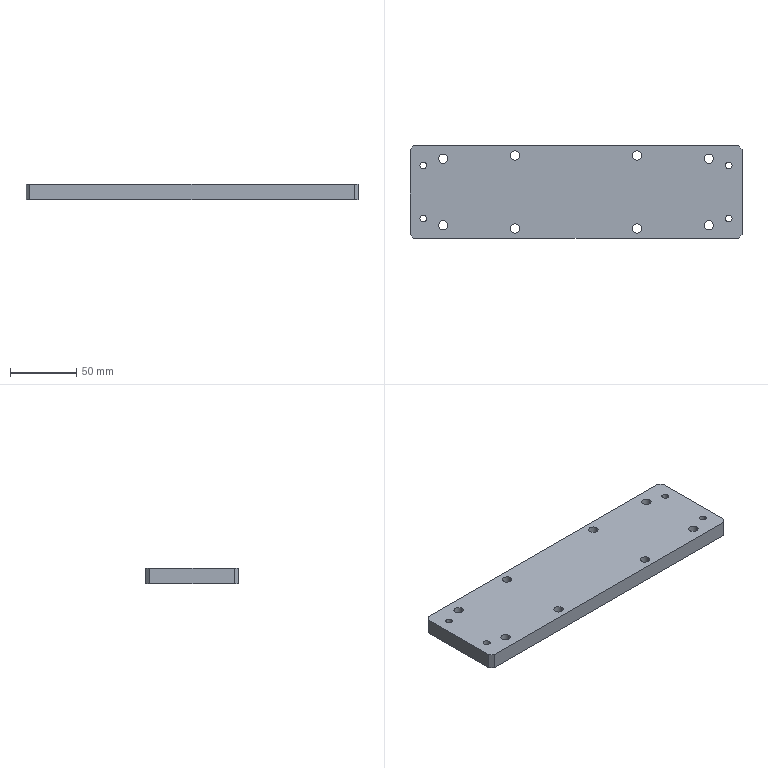Part | SolidWorks | features HoleWzd 3, Chamfer 1, Extrusion 1 | 1 solid | 34 faces | box 250 x 70 x 12 mm | volume 205147 mm3 | cylinder 24 | plane 10 | commonest cylinder face diameters 7 x16 5 x8
STEP:
#1=CARTESIAN_POINT('',(-42.5,27.5,12.));
#2=VERTEX_POINT('',#1);
#3=CARTESIAN_POINT('',(-49.5,27.5,12.));
#4=VERTEX_POINT('',#3);
#5=CARTESIAN_POINT('',(-46.,27.5,12.));
#6=DIRECTION('',(0.,0.,-1.));
#7=DIRECTION('',(-1.,0.,0.));
#8=AXIS2_PLACEMENT_3D('',#5,#6,#7);
#9=CIRCLE('',#8,3.5);
#10=EDGE_CURVE('',#2,#4,#9,.T.);
#11=ORIENTED_EDGE('',*,*,#10,.F.);
#12=CARTESIAN_POINT('',(-42.5,27.5,0.));
#13=VERTEX_POINT('',#12);
#14=CARTESIAN_POINT('',(-42.5,27.5,0.));
#15=DIRECTION('',(0.,0.,-1.));
#16=VECTOR('',#15,1000.);
#17=LINE('',#14,#16);
#18=EDGE_CURVE('',#2,#13,#17,.T.);
#19=ORIENTED_EDGE('',*,*,#18,.T.);
#20=CARTESIAN_POINT('',(-49.5,27.5,0.));
#21=VERTEX_POINT('',#20);
#22=CARTESIAN_POINT('',(-46.,27.5,0.));
#23=DIRECTION('',(0.,0.,-1.));
#24=DIRECTION('',(-1.,0.,0.));
#25=AXIS2_PLACEMENT_3D('',#22,#23,#24);
#26=CIRCLE('',#25,3.5);
#27=EDGE_CURVE('',#13,#21,#26,.T.);
#28=ORIENTED_EDGE('',*,*,#27,.T.);
#29=CARTESIAN_POINT('',(-49.5,27.5,0.));
#30=DIRECTION('',(0.,0.,-1.));
#31=VECTOR('',#30,1000.);
#32=LINE('',#29,#31);
#33=EDGE_CURVE('',#4,#21,#32,.T.);
#34=ORIENTED_EDGE('',*,*,#33,.F.);
#35=EDGE_LOOP('',(#11,#19,#28,#34));
#36=FACE_OUTER_BOUND('',#35,.T.);
#37=CARTESIAN_POINT('',(-46.,27.5,0.));
#38=DIRECTION('',(0.,0.,-1.));
#39=DIRECTION('',(-1.,0.,0.));
#40=AXIS2_PLACEMENT_3D('',#37,#38,#39);
#41=CYLINDRICAL_SURFACE('',#40,3.5);
#42=ADVANCED_FACE('',(#36),#41,.F.);
#43=CARTESIAN_POINT('',(-42.5,-27.5,12.));
#44=VERTEX_POINT('',#43);
#45=CARTESIAN_POINT('',(-49.5,-27.5,12.));
#46=VERTEX_POINT('',#45);
#47=CARTESIAN_POINT('',(-46.,-27.5,12.));
#48=DIRECTION('',(0.,0.,-1.));
#49=DIRECTION('',(-1.,0.,0.));
#50=AXIS2_PLACEMENT_3D('',#47,#48,#49);
#51=CIRCLE('',#50,3.5);
#52=EDGE_CURVE('',#44,#46,#51,.T.);
#53=ORIENTED_EDGE('',*,*,#52,.F.);
#54=CARTESIAN_POINT('',(-42.5,-27.5,0.));
#55=VERTEX_POINT('',#54);
#56=CARTESIAN_POINT('',(-42.5,-27.5,0.));
#57=DIRECTION('',(0.,0.,-1.));
#58=VECTOR('',#57,1000.);
#59=LINE('',#56,#58);
#60=EDGE_CURVE('',#44,#55,#59,.T.);
#61=ORIENTED_EDGE('',*,*,#60,.T.);
#62=CARTESIAN_POINT('',(-49.5,-27.5,0.));
#63=VERTEX_POINT('',#62);
#64=CARTESIAN_POINT('',(-46.,-27.5,0.));
#65=DIRECTION('',(0.,0.,-1.));
#66=DIRECTION('',(-1.,0.,0.));
#67=AXIS2_PLACEMENT_3D('',#64,#65,#66);
#68=CIRCLE('',#67,3.5);
#69=EDGE_CURVE('',#55,#63,#68,.T.);
#70=ORIENTED_EDGE('',*,*,#69,.T.);
#71=CARTESIAN_POINT('',(-49.5,-27.5,0.));
#72=DIRECTION('',(0.,0.,-1.));
#73=VECTOR('',#72,1000.);
#74=LINE('',#71,#73);
#75=EDGE_CURVE('',#46,#63,#74,.T.);
#76=ORIENTED_EDGE('',*,*,#75,.F.);
#77=EDGE_LOOP('',(#53,#61,#70,#76));
#78=FACE_OUTER_BOUND('',#77,.T.);
#79=CARTESIAN_POINT('',(-46.,-27.5,0.));
#80=DIRECTION('',(0.,0.,-1.));
#81=DIRECTION('',(-1.,0.,0.));
#82=AXIS2_PLACEMENT_3D('',#79,#80,#81);
#83=CYLINDRICAL_SURFACE('',#82,3.5);
#84=ADVANCED_FACE('',(#78),#83,.F.);
#85=CARTESIAN_POINT('',(49.5,27.5,12.));
#86=VERTEX_POINT('',#85);
#87=CARTESIAN_POINT('',(42.5,27.5,12.));
#88=VERTEX_POINT('',#87);
#89=CARTESIAN_POINT('',(46.,27.5,12.));
#90=DIRECTION('',(0.,0.,-1.));
#91=DIRECTION('',(-1.,0.,0.));
#92=AXIS2_PLACEMENT_3D('',#89,#90,#91);
#93=CIRCLE('',#92,3.5);
#94=EDGE_CURVE('',#86,#88,#93,.T.);
#95=ORIENTED_EDGE('',*,*,#94,.F.);
#96=CARTESIAN_POINT('',(49.5,27.5,0.));
#97=VERTEX_POINT('',#96);
#98=CARTESIAN_POINT('',(49.5,27.5,0.));
#99=DIRECTION('',(0.,0.,-1.));
#100=VECTOR('',#99,1000.);
#101=LINE('',#98,#100);
#102=EDGE_CURVE('',#86,#97,#101,.T.);
#103=ORIENTED_EDGE('',*,*,#102,.T.);
#104=CARTESIAN_POINT('',(42.5,27.5,0.));
#105=VERTEX_POINT('',#104);
#106=CARTESIAN_POINT('',(46.,27.5,0.));
#107=DIRECTION('',(0.,0.,-1.));
#108=DIRECTION('',(-1.,0.,0.));
#109=AXIS2_PLACEMENT_3D('',#106,#107,#108);
#110=CIRCLE('',#109,3.5);
#111=EDGE_CURVE('',#97,#105,#110,.T.);
#112=ORIENTED_EDGE('',*,*,#111,.T.);
#113=CARTESIAN_POINT('',(42.5,27.5,0.));
#114=DIRECTION('',(0.,0.,-1.));
#115=VECTOR('',#114,1000.);
#116=LINE('',#113,#115);
#117=EDGE_CURVE('',#88,#105,#116,.T.);
#118=ORIENTED_EDGE('',*,*,#117,.F.);
#119=EDGE_LOOP('',(#95,#103,#112,#118));
#120=FACE_OUTER_BOUND('',#119,.T.);
#121=CARTESIAN_POINT('',(46.,27.5,0.));
#122=DIRECTION('',(0.,0.,-1.));
#123=DIRECTION('',(-1.,0.,0.));
#124=AXIS2_PLACEMENT_3D('',#121,#122,#123);
#125=CYLINDRICAL_SURFACE('',#124,3.5);
#126=ADVANCED_FACE('',(#120),#125,.F.);
#127=CARTESIAN_POINT('',(49.5,-27.5,12.));
#128=VERTEX_POINT('',#127);
#129=CARTESIAN_POINT('',(42.5,-27.5,12.));
#130=VERTEX_POINT('',#129);
#131=CARTESIAN_POINT('',(46.,-27.5,12.));
#132=DIRECTION('',(0.,0.,-1.));
#133=DIRECTION('',(-1.,0.,0.));
#134=AXIS2_PLACEMENT_3D('',#131,#132,#133);
#135=CIRCLE('',#134,3.5);
#136=EDGE_CURVE('',#128,#130,#135,.T.);
#137=ORIENTED_EDGE('',*,*,#136,.F.);
#138=CARTESIAN_POINT('',(49.5,-27.5,0.));
#139=VERTEX_POINT('',#138);
#140=CARTESIAN_POINT('',(49.5,-27.5,0.));
#141=DIRECTION('',(0.,0.,-1.));
#142=VECTOR('',#141,1000.);
#143=LINE('',#140,#142);
#144=EDGE_CURVE('',#128,#139,#143,.T.);
#145=ORIENTED_EDGE('',*,*,#144,.T.);
#146=CARTESIAN_POINT('',(42.5,-27.5,0.));
#147=VERTEX_POINT('',#146);
#148=CARTESIAN_POINT('',(46.,-27.5,0.));
#149=DIRECTION('',(0.,0.,-1.));
#150=DIRECTION('',(-1.,0.,0.));
#151=AXIS2_PLACEMENT_3D('',#148,#149,#150);
#152=CIRCLE('',#151,3.5);
#153=EDGE_CURVE('',#139,#147,#152,.T.);
#154=ORIENTED_EDGE('',*,*,#153,.T.);
#155=CARTESIAN_POINT('',(42.5,-27.5,0.));
#156=DIRECTION('',(0.,0.,-1.));
#157=VECTOR('',#156,1000.);
#158=LINE('',#155,#157);
#159=EDGE_CURVE('',#130,#147,#158,.T.);
#160=ORIENTED_EDGE('',*,*,#159,.F.);
#161=EDGE_LOOP('',(#137,#145,#154,#160));
#162=FACE_OUTER_BOUND('',#161,.T.);
#163=CARTESIAN_POINT('',(46.,-27.5,0.));
#164=DIRECTION('',(0.,0.,-1.));
#165=DIRECTION('',(-1.,0.,0.));
#166=AXIS2_PLACEMENT_3D('',#163,#164,#165);
#167=CYLINDRICAL_SURFACE('',#166,3.5);
#168=ADVANCED_FACE('',(#162),#167,.F.);
#169=CARTESIAN_POINT('',(-112.5,-20.,12.));
#170=VERTEX_POINT('',#169);
#171=CARTESIAN_POINT('',(-117.5,-20.,12.));
#172=VERTEX_POINT('',#171);
#173=CARTESIAN_POINT('',(-115.,-20.,12.));
#174=DIRECTION('',(0.,0.,-1.));
#175=DIRECTION('',(-1.,0.,0.));
#176=AXIS2_PLACEMENT_3D('',#173,#174,#175);
#177=CIRCLE('',#176,2.5);
#178=EDGE_CURVE('',#170,#172,#177,.T.);
#179=ORIENTED_EDGE('',*,*,#178,.F.);
#180=CARTESIAN_POINT('',(-112.5,-20.,0.));
#181=VERTEX_POINT('',#180);
#182=CARTESIAN_POINT('',(-112.5,-20.,0.));
#183=DIRECTION('',(0.,0.,-1.));
#184=VECTOR('',#183,1000.);
#185=LINE('',#182,#184);
#186=EDGE_CURVE('',#170,#181,#185,.T.);
#187=ORIENTED_EDGE('',*,*,#186,.T.);
#188=CARTESIAN_POINT('',(-117.5,-20.,0.));
#189=VERTEX_POINT('',#188);
#190=CARTESIAN_POINT('',(-115.,-20.,0.));
#191=DIRECTION('',(0.,0.,-1.));
#192=DIRECTION('',(-1.,0.,0.));
#193=AXIS2_PLACEMENT_3D('',#190,#191,#192);
#194=CIRCLE('',#193,2.5);
#195=EDGE_CURVE('',#181,#189,#194,.T.);
#196=ORIENTED_EDGE('',*,*,#195,.T.);
#197=CARTESIAN_POINT('',(-117.5,-20.,0.));
#198=DIRECTION('',(0.,0.,-1.));
#199=VECTOR('',#198,1000.);
#200=LINE('',#197,#199);
#201=EDGE_CURVE('',#172,#189,#200,.T.);
#202=ORIENTED_EDGE('',*,*,#201,.F.);
#203=EDGE_LOOP('',(#179,#187,#196,#202));
#204=FACE_OUTER_BOUND('',#203,.T.);
#205=CARTESIAN_POINT('',(-115.,-20.,0.));
#206=DIRECTION('',(0.,0.,-1.));
#207=DIRECTION('',(-1.,0.,0.));
#208=AXIS2_PLACEMENT_3D('',#205,#206,#207);
#209=CYLINDRICAL_SURFACE('',#208,2.5);
#210=ADVANCED_FACE('',(#204),#209,.F.);
#211=CARTESIAN_POINT('',(-112.5,20.,12.));
#212=VERTEX_POINT('',#211);
#213=CARTESIAN_POINT('',(-117.5,20.,12.));
#214=VERTEX_POINT('',#213);
#215=CARTESIAN_POINT('',(-115.,20.,12.));
#216=DIRECTION('',(0.,0.,-1.));
#217=DIRECTION('',(-1.,0.,0.));
#218=AXIS2_PLACEMENT_3D('',#215,#216,#217);
#219=CIRCLE('',#218,2.5);
#220=EDGE_CURVE('',#212,#214,#219,.T.);
#221=ORIENTED_EDGE('',*,*,#220,.F.);
#222=CARTESIAN_POINT('',(-112.5,20.,0.));
#223=VERTEX_POINT('',#222);
#224=CARTESIAN_POINT('',(-112.5,20.,0.));
#225=DIRECTION('',(0.,0.,-1.));
#226=VECTOR('',#225,1000.);
#227=LINE('',#224,#226);
#228=EDGE_CURVE('',#212,#223,#227,.T.);
#229=ORIENTED_EDGE('',*,*,#228,.T.);
#230=CARTESIAN_POINT('',(-117.5,20.,0.));
#231=VERTEX_POINT('',#230);
#232=CARTESIAN_POINT('',(-115.,20.,0.));
#233=DIRECTION('',(0.,0.,-1.));
#234=DIRECTION('',(-1.,0.,0.));
#235=AXIS2_PLACEMENT_3D('',#232,#233,#234);
#236=CIRCLE('',#235,2.5);
#237=EDGE_CURVE('',#223,#231,#236,.T.);
#238=ORIENTED_EDGE('',*,*,#237,.T.);
#239=CARTESIAN_POINT('',(-117.5,20.,0.));
#240=DIRECTION('',(0.,0.,-1.));
#241=VECTOR('',#240,1000.);
#242=LINE('',#239,#241);
#243=EDGE_CURVE('',#214,#231,#242,.T.);
#244=ORIENTED_EDGE('',*,*,#243,.F.);
#245=EDGE_LOOP('',(#221,#229,#238,#244));
#246=FACE_OUTER_BOUND('',#245,.T.);
#247=CARTESIAN_POINT('',(-115.,20.,0.));
#248=DIRECTION('',(0.,0.,-1.));
#249=DIRECTION('',(-1.,0.,0.));
#250=AXIS2_PLACEMENT_3D('',#247,#248,#249);
#251=CYLINDRICAL_SURFACE('',#250,2.5);
#252=ADVANCED_FACE('',(#246),#251,.F.);
#253=CARTESIAN_POINT('',(117.5,20.,12.));
#254=VERTEX_POINT('',#253);
#255=CARTESIAN_POINT('',(112.5,20.,12.));
#256=VERTEX_POINT('',#255);
#257=CARTESIAN_POINT('',(115.,20.,12.));
#258=DIRECTION('',(0.,0.,-1.));
#259=DIRECTION('',(-1.,0.,0.));
#260=AXIS2_PLACEMENT_3D('',#257,#258,#259);
#261=CIRCLE('',#260,2.5);
#262=EDGE_CURVE('',#254,#256,#261,.T.);
#263=ORIENTED_EDGE('',*,*,#262,.F.);
#264=CARTESIAN_POINT('',(117.5,20.,0.));
#265=VERTEX_POINT('',#264);
#266=CARTESIAN_POINT('',(117.5,20.,0.));
#267=DIRECTION('',(0.,0.,-1.));
#268=VECTOR('',#267,1000.);
#269=LINE('',#266,#268);
#270=EDGE_CURVE('',#254,#265,#269,.T.);
#271=ORIENTED_EDGE('',*,*,#270,.T.);
#272=CARTESIAN_POINT('',(112.5,20.,0.));
#273=VERTEX_POINT('',#272);
#274=CARTESIAN_POINT('',(115.,20.,0.));
#275=DIRECTION('',(0.,0.,-1.));
#276=DIRECTION('',(-1.,0.,0.));
#277=AXIS2_PLACEMENT_3D('',#274,#275,#276);
#278=CIRCLE('',#277,2.5);
#279=EDGE_CURVE('',#265,#273,#278,.T.);
#280=ORIENTED_EDGE('',*,*,#279,.T.);
#281=CARTESIAN_POINT('',(112.5,20.,0.));
#282=DIRECTION('',(0.,0.,-1.));
#283=VECTOR('',#282,1000.);
#284=LINE('',#281,#283);
#285=EDGE_CURVE('',#256,#273,#284,.T.);
#286=ORIENTED_EDGE('',*,*,#285,.F.);
#287=EDGE_LOOP('',(#263,#271,#280,#286));
#288=FACE_OUTER_BOUND('',#287,.T.);
#289=CARTESIAN_POINT('',(115.,20.,0.));
#290=DIRECTION('',(0.,0.,-1.));
#291=DIRECTION('',(-1.,0.,0.));
#292=AXIS2_PLACEMENT_3D('',#289,#290,#291);
#293=CYLINDRICAL_SURFACE('',#292,2.5);
#294=ADVANCED_FACE('',(#288),#293,.F.);
#295=CARTESIAN_POINT('',(117.5,-20.,12.));
#296=VERTEX_POINT('',#295);
#297=CARTESIAN_POINT('',(112.5,-20.,12.));
#298=VERTEX_POINT('',#297);
#299=CARTESIAN_POINT('',(115.,-20.,12.));
#300=DIRECTION('',(0.,0.,-1.));
#301=DIRECTION('',(-1.,0.,0.));
#302=AXIS2_PLACEMENT_3D('',#299,#300,#301);
#303=CIRCLE('',#302,2.5);
#304=EDGE_CURVE('',#296,#298,#303,.T.);
#305=ORIENTED_EDGE('',*,*,#304,.F.);
#306=CARTESIAN_POINT('',(117.5,-20.,0.));
#307=VERTEX_POINT('',#306);
#308=CARTESIAN_POINT('',(117.5,-20.,0.));
#309=DIRECTION('',(0.,0.,-1.));
#310=VECTOR('',#309,1000.);
#311=LINE('',#308,#310);
#312=EDGE_CURVE('',#296,#307,#311,.T.);
#313=ORIENTED_EDGE('',*,*,#312,.T.);
#314=CARTESIAN_POINT('',(112.5,-20.,0.));
#315=VERTEX_POINT('',#314);
#316=CARTESIAN_POINT('',(115.,-20.,0.));
#317=DIRECTION('',(0.,0.,-1.));
#318=DIRECTION('',(-1.,0.,0.));
#319=AXIS2_PLACEMENT_3D('',#316,#317,#318);
#320=CIRCLE('',#319,2.5);
#321=EDGE_CURVE('',#307,#315,#320,.T.);
#322=ORIENTED_EDGE('',*,*,#321,.T.);
#323=CARTESIAN_POINT('',(112.5,-20.,0.));
#324=DIRECTION('',(0.,0.,-1.));
#325=VECTOR('',#324,1000.);
#326=LINE('',#323,#325);
#327=EDGE_CURVE('',#298,#315,#326,.T.);
#328=ORIENTED_EDGE('',*,*,#327,.F.);
#329=EDGE_LOOP('',(#305,#313,#322,#328));
#330=FACE_OUTER_BOUND('',#329,.T.);
#331=CARTESIAN_POINT('',(115.,-20.,0.));
#332=DIRECTION('',(0.,0.,-1.));
#333=DIRECTION('',(-1.,0.,0.));
#334=AXIS2_PLACEMENT_3D('',#331,#332,#333);
#335=CYLINDRICAL_SURFACE('',#334,2.5);
#336=ADVANCED_FACE('',(#330),#335,.F.);
#337=CARTESIAN_POINT('',(-96.5,-25.,12.));
#338=VERTEX_POINT('',#337);
#339=CARTESIAN_POINT('',(-103.5,-25.,12.));
#340=VERTEX_POINT('',#339);
#341=CARTESIAN_POINT('',(-100.,-25.,12.));
#342=DIRECTION('',(0.,0.,-1.));
#343=DIRECTION('',(-1.,0.,0.));
#344=AXIS2_PLACEMENT_3D('',#341,#342,#343);
#345=CIRCLE('',#344,3.5);
#346=EDGE_CURVE('',#338,#340,#345,.T.);
#347=ORIENTED_EDGE('',*,*,#346,.F.);
#348=CARTESIAN_POINT('',(-96.5,-25.,0.));
#349=VERTEX_POINT('',#348);
#350=CARTESIAN_POINT('',(-96.5,-25.,0.));
#351=DIRECTION('',(0.,0.,-1.));
#352=VECTOR('',#351,1000.);
#353=LINE('',#350,#352);
#354=EDGE_CURVE('',#338,#349,#353,.T.);
#355=ORIENTED_EDGE('',*,*,#354,.T.);
#356=CARTESIAN_POINT('',(-103.5,-25.,0.));
#357=VERTEX_POINT('',#356);
#358=CARTESIAN_POINT('',(-100.,-25.,0.));
#359=DIRECTION('',(0.,0.,-1.));
#360=DIRECTION('',(-1.,0.,0.));
#361=AXIS2_PLACEMENT_3D('',#358,#359,#360);
#362=CIRCLE('',#361,3.5);
#363=EDGE_CURVE('',#349,#357,#362,.T.);
#364=ORIENTED_EDGE('',*,*,#363,.T.);
#365=CARTESIAN_POINT('',(-103.5,-25.,0.));
#366=DIRECTION('',(0.,0.,-1.));
#367=VECTOR('',#366,1000.);
#368=LINE('',#365,#367);
#369=EDGE_CURVE('',#340,#357,#368,.T.);
#370=ORIENTED_EDGE('',*,*,#369,.F.);
#371=EDGE_LOOP('',(#347,#355,#364,#370));
#372=FACE_OUTER_BOUND('',#371,.T.);
#373=CARTESIAN_POINT('',(-100.,-25.,0.));
#374=DIRECTION('',(0.,0.,-1.));
#375=DIRECTION('',(-1.,0.,0.));
#376=AXIS2_PLACEMENT_3D('',#373,#374,#375);
#377=CYLINDRICAL_SURFACE('',#376,3.5);
#378=ADVANCED_FACE('',(#372),#377,.F.);
#379=CARTESIAN_POINT('',(-96.5,25.,12.));
#380=VERTEX_POINT('',#379);
#381=CARTESIAN_POINT('',(-103.5,25.,12.));
#382=VERTEX_POINT('',#381);
#383=CARTESIAN_POINT('',(-100.,25.,12.));
#384=DIRECTION('',(0.,0.,-1.));
#385=DIRECTION('',(-1.,0.,0.));
#386=AXIS2_PLACEMENT_3D('',#383,#384,#385);
#387=CIRCLE('',#386,3.5);
#388=EDGE_CURVE('',#380,#382,#387,.T.);
#389=ORIENTED_EDGE('',*,*,#388,.F.);
#390=CARTESIAN_POINT('',(-96.5,25.,0.));
#391=VERTEX_POINT('',#390);
#392=CARTESIAN_POINT('',(-96.5,25.,0.));
#393=DIRECTION('',(0.,0.,-1.));
#394=VECTOR('',#393,1000.);
#395=LINE('',#392,#394);
#396=EDGE_CURVE('',#380,#391,#395,.T.);
#397=ORIENTED_EDGE('',*,*,#396,.T.);
#398=CARTESIAN_POINT('',(-103.5,25.,0.));
#399=VERTEX_POINT('',#398);
#400=CARTESIAN_POINT('',(-100.,25.,0.));
#401=DIRECTION('',(0.,0.,-1.));
#402=DIRECTION('',(-1.,0.,0.));
#403=AXIS2_PLACEMENT_3D('',#400,#401,#402);
#404=CIRCLE('',#403,3.5);
#405=EDGE_CURVE('',#391,#399,#404,.T.);
#406=ORIENTED_EDGE('',*,*,#405,.T.);
#407=CARTESIAN_POINT('',(-103.5,25.,0.));
#408=DIRECTION('',(0.,0.,-1.));
#409=VECTOR('',#408,1000.);
#410=LINE('',#407,#409);
#411=EDGE_CURVE('',#382,#399,#410,.T.);
#412=ORIENTED_EDGE('',*,*,#411,.F.);
#413=EDGE_LOOP('',(#389,#397,#406,#412));
#414=FACE_OUTER_BOUND('',#413,.T.);
#415=CARTESIAN_POINT('',(-100.,25.,0.));
#416=DIRECTION('',(0.,0.,-1.));
#417=DIRECTION('',(-1.,0.,0.));
#418=AXIS2_PLACEMENT_3D('',#415,#416,#417);
#419=CYLINDRICAL_SURFACE('',#418,3.5);
#420=ADVANCED_FACE('',(#414),#419,.F.);
#421=CARTESIAN_POINT('',(103.5,25.,12.));
#422=VERTEX_POINT('',#421);
#423=CARTESIAN_POINT('',(96.5,25.,12.));
#424=VERTEX_POINT('',#423);
#425=CARTESIAN_POINT('',(100.,25.,12.));
#426=DIRECTION('',(0.,0.,-1.));
#427=DIRECTION('',(-1.,0.,0.));
#428=AXIS2_PLACEMENT_3D('',#425,#426,#427);
#429=CIRCLE('',#428,3.5);
#430=EDGE_CURVE('',#422,#424,#429,.T.);
#431=ORIENTED_EDGE('',*,*,#430,.F.);
#432=CARTESIAN_POINT('',(103.5,25.,0.));
#433=VERTEX_POINT('',#432);
#434=CARTESIAN_POINT('',(103.5,25.,0.));
#435=DIRECTION('',(0.,0.,-1.));
#436=VECTOR('',#435,1000.);
#437=LINE('',#434,#436);
#438=EDGE_CURVE('',#422,#433,#437,.T.);
#439=ORIENTED_EDGE('',*,*,#438,.T.);
#440=CARTESIAN_POINT('',(96.5,25.,0.));
#441=VERTEX_POINT('',#440);
#442=CARTESIAN_POINT('',(100.,25.,0.));
#443=DIRECTION('',(0.,0.,-1.));
#444=DIRECTION('',(-1.,0.,0.));
#445=AXIS2_PLACEMENT_3D('',#442,#443,#444);
#446=CIRCLE('',#445,3.5);
#447=EDGE_CURVE('',#433,#441,#446,.T.);
#448=ORIENTED_EDGE('',*,*,#447,.T.);
#449=CARTESIAN_POINT('',(96.5,25.,0.));
#450=DIRECTION('',(0.,0.,-1.));
#451=VECTOR('',#450,1000.);
#452=LINE('',#449,#451);
#453=EDGE_CURVE('',#424,#441,#452,.T.);
#454=ORIENTED_EDGE('',*,*,#453,.F.);
#455=EDGE_LOOP('',(#431,#439,#448,#454));
#456=FACE_OUTER_BOUND('',#455,.T.);
#457=CARTESIAN_POINT('',(100.,25.,0.));
#458=DIRECTION('',(0.,0.,-1.));
#459=DIRECTION('',(-1.,0.,0.));
#460=AXIS2_PLACEMENT_3D('',#457,#458,#459);
#461=CYLINDRICAL_SURFACE('',#460,3.5);
#462=ADVANCED_FACE('',(#456),#461,.F.);
#463=CARTESIAN_POINT('',(103.5,-25.,12.));
#464=VERTEX_POINT('',#463);
#465=CARTESIAN_POINT('',(96.5,-25.,12.));
#466=VERTEX_POINT('',#465);
#467=CARTESIAN_POINT('',(100.,-25.,12.));
#468=DIRECTION('',(0.,0.,-1.));
#469=DIRECTION('',(-1.,0.,0.));
#470=AXIS2_PLACEMENT_3D('',#467,#468,#469);
#471=CIRCLE('',#470,3.5);
#472=EDGE_CURVE('',#464,#466,#471,.T.);
#473=ORIENTED_EDGE('',*,*,#472,.F.);
#474=CARTESIAN_POINT('',(103.5,-25.,0.));
#475=VERTEX_POINT('',#474);
#476=CARTESIAN_POINT('',(103.5,-25.,0.));
#477=DIRECTION('',(0.,0.,-1.));
#478=VECTOR('',#477,1000.);
#479=LINE('',#476,#478);
#480=EDGE_CURVE('',#464,#475,#479,.T.);
#481=ORIENTED_EDGE('',*,*,#480,.T.);
#482=CARTESIAN_POINT('',(96.5,-25.,0.));
#483=VERTEX_POINT('',#482);
#484=CARTESIAN_POINT('',(100.,-25.,0.));
#485=DIRECTION('',(0.,0.,-1.));
#486=DIRECTION('',(-1.,0.,0.));
#487=AXIS2_PLACEMENT_3D('',#484,#485,#486);
#488=CIRCLE('',#487,3.5);
#489=EDGE_CURVE('',#475,#483,#488,.T.);
#490=ORIENTED_EDGE('',*,*,#489,.T.);
#491=CARTESIAN_POINT('',(96.5,-25.,0.));
#492=DIRECTION('',(0.,0.,-1.));
#493=VECTOR('',#492,1000.);
#494=LINE('',#491,#493);
#495=EDGE_CURVE('',#466,#483,#494,.T.);
#496=ORIENTED_EDGE('',*,*,#495,.F.);
#497=EDGE_LOOP('',(#473,#481,#490,#496));
#498=FACE_OUTER_BOUND('',#497,.T.);
#499=CARTESIAN_POINT('',(100.,-25.,0.));
#500=DIRECTION('',(0.,0.,-1.));
#501=DIRECTION('',(-1.,0.,0.));
#502=AXIS2_PLACEMENT_3D('',#499,#500,#501);
#503=CYLINDRICAL_SURFACE('',#502,3.5);
#504=ADVANCED_FACE('',(#498),#503,.F.);
#505=CARTESIAN_POINT('',(125.,-32.,12.));
#506=VERTEX_POINT('',#505);
#507=CARTESIAN_POINT('',(125.,32.,12.));
#508=VERTEX_POINT('',#507);
#509=CARTESIAN_POINT('',(125.,35.,12.));
#510=DIRECTION('',(0.,1.,0.));
#511=VECTOR('',#510,1000.);
#512=LINE('',#509,#511);
#513=EDGE_CURVE('',#506,#508,#512,.T.);
#514=ORIENTED_EDGE('',*,*,#513,.F.);
#515=CARTESIAN_POINT('',(125.,-32.,0.));
#516=VERTEX_POINT('',#515);
#517=CARTESIAN_POINT('',(125.,-32.,12.));
#518=DIRECTION('',(0.,0.,-1.));
#519=VECTOR('',#518,1000.);
#520=LINE('',#517,#519);
#521=EDGE_CURVE('',#506,#516,#520,.T.);
#522=ORIENTED_EDGE('',*,*,#521,.T.);
#523=CARTESIAN_POINT('',(125.,32.,0.));
#524=VERTEX_POINT('',#523);
#525=CARTESIAN_POINT('',(125.,35.,0.));
#526=DIRECTION('',(0.,1.,0.));
#527=VECTOR('',#526,1000.);
#528=LINE('',#525,#527);
#529=EDGE_CURVE('',#516,#524,#528,.T.);
#530=ORIENTED_EDGE('',*,*,#529,.T.);
#531=CARTESIAN_POINT('',(125.,32.,12.));
#532=DIRECTION('',(0.,0.,1.));
#533=VECTOR('',#532,1000.);
#534=LINE('',#531,#533);
#535=EDGE_CURVE('',#524,#508,#534,.T.);
#536=ORIENTED_EDGE('',*,*,#535,.T.);
#537=EDGE_LOOP('',(#514,#522,#530,#536));
#538=FACE_OUTER_BOUND('',#537,.T.);
#539=CARTESIAN_POINT('',(125.,35.,12.));
#540=DIRECTION('',(-1.,0.,0.));
#541=DIRECTION('',(0.,0.,1.));
#542=AXIS2_PLACEMENT_3D('',#539,#540,#541);
#543=PLANE('',#542);
#544=ADVANCED_FACE('',(#538),#543,.F.);
#545=CARTESIAN_POINT('',(122.,35.,12.));
#546=VERTEX_POINT('',#545);
#547=CARTESIAN_POINT('',(-122.,35.,12.));
#548=VERTEX_POINT('',#547);
#549=CARTESIAN_POINT('',(-125.,35.,12.));
#550=DIRECTION('',(-1.,0.,0.));
#551=VECTOR('',#550,1000.);
#552=LINE('',#549,#551);
#553=EDGE_CURVE('',#546,#548,#552,.T.);
#554=ORIENTED_EDGE('',*,*,#553,.F.);
#555=CARTESIAN_POINT('',(122.,35.,0.));
#556=VERTEX_POINT('',#555);
#557=CARTESIAN_POINT('',(122.,35.,12.));
#558=DIRECTION('',(0.,0.,-1.));
#559=VECTOR('',#558,1000.);
#560=LINE('',#557,#559);
#561=EDGE_CURVE('',#546,#556,#560,.T.);
#562=ORIENTED_EDGE('',*,*,#561,.T.);
#563=CARTESIAN_POINT('',(-122.,35.,0.));
#564=VERTEX_POINT('',#563);
#565=CARTESIAN_POINT('',(-125.,35.,0.));
#566=DIRECTION('',(-1.,0.,0.));
#567=VECTOR('',#566,1000.);
#568=LINE('',#565,#567);
#569=EDGE_CURVE('',#556,#564,#568,.T.);
#570=ORIENTED_EDGE('',*,*,#569,.T.);
#571=CARTESIAN_POINT('',(-122.,35.,12.));
#572=DIRECTION('',(0.,0.,1.));
#573=VECTOR('',#572,1000.);
#574=LINE('',#571,#573);
#575=EDGE_CURVE('',#564,#548,#574,.T.);
#576=ORIENTED_EDGE('',*,*,#575,.T.);
#577=EDGE_LOOP('',(#554,#562,#570,#576));
#578=FACE_OUTER_BOUND('',#577,.T.);
#579=CARTESIAN_POINT('',(-125.,35.,12.));
#580=DIRECTION('',(0.,-1.,0.));
#581=DIRECTION('',(0.,0.,-1.));
#582=AXIS2_PLACEMENT_3D('',#579,#580,#581);
#583=PLANE('',#582);
#584=ADVANCED_FACE('',(#578),#583,.F.);
#585=CARTESIAN_POINT('',(-125.,32.,0.));
#586=VERTEX_POINT('',#585);
#587=CARTESIAN_POINT('',(-125.,-32.,0.));
#588=VERTEX_POINT('',#587);
#589=CARTESIAN_POINT('',(-125.,35.,0.));
#590=DIRECTION('',(0.,-1.,0.));
#591=VECTOR('',#590,1000.);
#592=LINE('',#589,#591);
#593=EDGE_CURVE('',#586,#588,#592,.T.);
#594=ORIENTED_EDGE('',*,*,#593,.T.);
#595=CARTESIAN_POINT('',(-125.,-32.,12.));
#596=VERTEX_POINT('',#595);
#597=CARTESIAN_POINT('',(-125.,-32.,12.));
#598=DIRECTION('',(0.,0.,1.));
#599=VECTOR('',#598,1000.);
#600=LINE('',#597,#599);
#601=EDGE_CURVE('',#588,#596,#600,.T.);
#602=ORIENTED_EDGE('',*,*,#601,.T.);
#603=CARTESIAN_POINT('',(-125.,32.,12.));
#604=VERTEX_POINT('',#603);
#605=CARTESIAN_POINT('',(-125.,35.,12.));
#606=DIRECTION('',(0.,-1.,0.));
#607=VECTOR('',#606,1000.);
#608=LINE('',#605,#607);
#609=EDGE_CURVE('',#604,#596,#608,.T.);
#610=ORIENTED_EDGE('',*,*,#609,.F.);
#611=CARTESIAN_POINT('',(-125.,32.,12.));
#612=DIRECTION('',(0.,0.,-1.));
#613=VECTOR('',#612,1000.);
#614=LINE('',#611,#613);
#615=EDGE_CURVE('',#604,#586,#614,.T.);
#616=ORIENTED_EDGE('',*,*,#615,.T.);
#617=EDGE_LOOP('',(#594,#602,#610,#616));
#618=FACE_OUTER_BOUND('',#617,.T.);
#619=CARTESIAN_POINT('',(-125.,35.,12.));
#620=DIRECTION('',(1.,0.,0.));
#621=DIRECTION('',(0.,0.,-1.));
#622=AXIS2_PLACEMENT_3D('',#619,#620,#621);
#623=PLANE('',#622);
#624=ADVANCED_FACE('',(#618),#623,.F.);
#625=CARTESIAN_POINT('',(-122.,-35.,0.));
#626=VERTEX_POINT('',#625);
#627=CARTESIAN_POINT('',(122.,-35.,0.));
#628=VERTEX_POINT('',#627);
#629=CARTESIAN_POINT('',(-125.,-35.,0.));
#630=DIRECTION('',(1.,0.,0.));
#631=VECTOR('',#630,1000.);
#632=LINE('',#629,#631);
#633=EDGE_CURVE('',#626,#628,#632,.T.);
#634=ORIENTED_EDGE('',*,*,#633,.T.);
#635=CARTESIAN_POINT('',(122.,-35.,12.));
#636=VERTEX_POINT('',#635);
#637=CARTESIAN_POINT('',(122.,-35.,12.));
#638=DIRECTION('',(0.,0.,1.));
#639=VECTOR('',#638,1000.);
#640=LINE('',#637,#639);
#641=EDGE_CURVE('',#628,#636,#640,.T.);
#642=ORIENTED_EDGE('',*,*,#641,.T.);
#643=CARTESIAN_POINT('',(-122.,-35.,12.));
#644=VERTEX_POINT('',#643);
#645=CARTESIAN_POINT('',(-125.,-35.,12.));
#646=DIRECTION('',(1.,0.,0.));
#647=VECTOR('',#646,1000.);
#648=LINE('',#645,#647);
#649=EDGE_CURVE('',#644,#636,#648,.T.);
#650=ORIENTED_EDGE('',*,*,#649,.F.);
#651=CARTESIAN_POINT('',(-122.,-35.,12.));
#652=DIRECTION('',(0.,0.,-1.));
#653=VECTOR('',#652,1000.);
#654=LINE('',#651,#653);
#655=EDGE_CURVE('',#644,#626,#654,.T.);
#656=ORIENTED_EDGE('',*,*,#655,.T.);
#657=EDGE_LOOP('',(#634,#642,#650,#656));
#658=FACE_OUTER_BOUND('',#657,.T.);
#659=CARTESIAN_POINT('',(-125.,-35.,12.));
#660=DIRECTION('',(0.,1.,0.));
#661=DIRECTION('',(0.,0.,1.));
#662=AXIS2_PLACEMENT_3D('',#659,#660,#661);
#663=PLANE('',#662);
#664=ADVANCED_FACE('',(#658),#663,.F.);
#665=CARTESIAN_POINT('',(-46.,27.5,12.));
#666=DIRECTION('',(0.,0.,-1.));
#667=DIRECTION('',(-1.,0.,0.));
#668=AXIS2_PLACEMENT_3D('',#665,#666,#667);
#669=CIRCLE('',#668,3.5);
#670=EDGE_CURVE('',#4,#2,#669,.T.);
#671=ORIENTED_EDGE('',*,*,#670,.T.);
#672=ORIENTED_EDGE('',*,*,#10,.T.);
#673=EDGE_LOOP('',(#671,#672));
#674=FACE_BOUND('',#673,.T.);
#675=CARTESIAN_POINT('',(-46.,-27.5,12.));
#676=DIRECTION('',(0.,0.,-1.));
#677=DIRECTION('',(-1.,0.,0.));
#678=AXIS2_PLACEMENT_3D('',#675,#676,#677);
#679=CIRCLE('',#678,3.5);
#680=EDGE_CURVE('',#46,#44,#679,.T.);
#681=ORIENTED_EDGE('',*,*,#680,.T.);
#682=ORIENTED_EDGE('',*,*,#52,.T.);
#683=EDGE_LOOP('',(#681,#682));
#684=FACE_BOUND('',#683,.T.);
#685=CARTESIAN_POINT('',(46.,27.5,12.));
#686=DIRECTION('',(0.,0.,-1.));
#687=DIRECTION('',(-1.,0.,0.));
#688=AXIS2_PLACEMENT_3D('',#685,#686,#687);
#689=CIRCLE('',#688,3.5);
#690=EDGE_CURVE('',#88,#86,#689,.T.);
#691=ORIENTED_EDGE('',*,*,#690,.T.);
#692=ORIENTED_EDGE('',*,*,#94,.T.);
#693=EDGE_LOOP('',(#691,#692));
#694=FACE_BOUND('',#693,.T.);
#695=CARTESIAN_POINT('',(46.,-27.5,12.));
#696=DIRECTION('',(0.,0.,-1.));
#697=DIRECTION('',(-1.,0.,0.));
#698=AXIS2_PLACEMENT_3D('',#695,#696,#697);
#699=CIRCLE('',#698,3.5);
#700=EDGE_CURVE('',#130,#128,#699,.T.);
#701=ORIENTED_EDGE('',*,*,#700,.T.);
#702=ORIENTED_EDGE('',*,*,#136,.T.);
#703=EDGE_LOOP('',(#701,#702));
#704=FACE_BOUND('',#703,.T.);
#705=CARTESIAN_POINT('',(-115.,-20.,12.));
#706=DIRECTION('',(0.,0.,-1.));
#707=DIRECTION('',(-1.,0.,0.));
#708=AXIS2_PLACEMENT_3D('',#705,#706,#707);
#709=CIRCLE('',#708,2.5);
#710=EDGE_CURVE('',#172,#170,#709,.T.);
#711=ORIENTED_EDGE('',*,*,#710,.T.);
#712=ORIENTED_EDGE('',*,*,#178,.T.);
#713=EDGE_LOOP('',(#711,#712));
#714=FACE_BOUND('',#713,.T.);
#715=CARTESIAN_POINT('',(-115.,20.,12.));
#716=DIRECTION('',(0.,0.,-1.));
#717=DIRECTION('',(-1.,0.,0.));
#718=AXIS2_PLACEMENT_3D('',#715,#716,#717);
#719=CIRCLE('',#718,2.5);
#720=EDGE_CURVE('',#214,#212,#719,.T.);
#721=ORIENTED_EDGE('',*,*,#720,.T.);
#722=ORIENTED_EDGE('',*,*,#220,.T.);
#723=EDGE_LOOP('',(#721,#722));
#724=FACE_BOUND('',#723,.T.);
#725=CARTESIAN_POINT('',(115.,20.,12.));
#726=DIRECTION('',(0.,0.,-1.));
#727=DIRECTION('',(-1.,0.,0.));
#728=AXIS2_PLACEMENT_3D('',#725,#726,#727);
#729=CIRCLE('',#728,2.5);
#730=EDGE_CURVE('',#256,#254,#729,.T.);
#731=ORIENTED_EDGE('',*,*,#730,.T.);
#732=ORIENTED_EDGE('',*,*,#262,.T.);
#733=EDGE_LOOP('',(#731,#732));
#734=FACE_BOUND('',#733,.T.);
#735=CARTESIAN_POINT('',(115.,-20.,12.));
#736=DIRECTION('',(0.,0.,-1.));
#737=DIRECTION('',(-1.,0.,0.));
#738=AXIS2_PLACEMENT_3D('',#735,#736,#737);
#739=CIRCLE('',#738,2.5);
#740=EDGE_CURVE('',#298,#296,#739,.T.);
#741=ORIENTED_EDGE('',*,*,#740,.T.);
#742=ORIENTED_EDGE('',*,*,#304,.T.);
#743=EDGE_LOOP('',(#741,#742));
#744=FACE_BOUND('',#743,.T.);
#745=CARTESIAN_POINT('',(-100.,-25.,12.));
#746=DIRECTION('',(0.,0.,-1.));
#747=DIRECTION('',(-1.,0.,0.));
#748=AXIS2_PLACEMENT_3D('',#745,#746,#747);
#749=CIRCLE('',#748,3.5);
#750=EDGE_CURVE('',#340,#338,#749,.T.);
#751=ORIENTED_EDGE('',*,*,#750,.T.);
#752=ORIENTED_EDGE('',*,*,#346,.T.);
#753=EDGE_LOOP('',(#751,#752));
#754=FACE_BOUND('',#753,.T.);
#755=CARTESIAN_POINT('',(-100.,25.,12.));
#756=DIRECTION('',(0.,0.,-1.));
#757=DIRECTION('',(-1.,0.,0.));
#758=AXIS2_PLACEMENT_3D('',#755,#756,#757);
#759=CIRCLE('',#758,3.5);
#760=EDGE_CURVE('',#382,#380,#759,.T.);
#761=ORIENTED_EDGE('',*,*,#760,.T.);
#762=ORIENTED_EDGE('',*,*,#388,.T.);
#763=EDGE_LOOP('',(#761,#762));
#764=FACE_BOUND('',#763,.T.);
#765=CARTESIAN_POINT('',(100.,25.,12.));
#766=DIRECTION('',(0.,0.,-1.));
#767=DIRECTION('',(-1.,0.,0.));
#768=AXIS2_PLACEMENT_3D('',#765,#766,#767);
#769=CIRCLE('',#768,3.5);
#770=EDGE_CURVE('',#424,#422,#769,.T.);
#771=ORIENTED_EDGE('',*,*,#770,.T.);
#772=ORIENTED_EDGE('',*,*,#430,.T.);
#773=EDGE_LOOP('',(#771,#772));
#774=FACE_BOUND('',#773,.T.);
#775=CARTESIAN_POINT('',(100.,-25.,12.));
#776=DIRECTION('',(0.,0.,-1.));
#777=DIRECTION('',(-1.,0.,0.));
#778=AXIS2_PLACEMENT_3D('',#775,#776,#777);
#779=CIRCLE('',#778,3.5);
#780=EDGE_CURVE('',#466,#464,#779,.T.);
#781=ORIENTED_EDGE('',*,*,#780,.T.);
#782=ORIENTED_EDGE('',*,*,#472,.T.);
#783=EDGE_LOOP('',(#781,#782));
#784=FACE_BOUND('',#783,.T.);
#785=ORIENTED_EDGE('',*,*,#649,.T.);
#786=CARTESIAN_POINT('',(78.5,-78.5,12.));
#787=DIRECTION('',(0.7071,0.7071,0.));
#788=VECTOR('',#787,1000.);
#789=LINE('',#786,#788);
#790=EDGE_CURVE('',#636,#506,#789,.T.);
#791=ORIENTED_EDGE('',*,*,#790,.T.);
#792=ORIENTED_EDGE('',*,*,#513,.T.);
#793=CARTESIAN_POINT('',(78.5,78.5,12.));
#794=DIRECTION('',(-0.7071,0.7071,0.));
#795=VECTOR('',#794,1000.);
#796=LINE('',#793,#795);
#797=EDGE_CURVE('',#508,#546,#796,.T.);
#798=ORIENTED_EDGE('',*,*,#797,.T.);
#799=ORIENTED_EDGE('',*,*,#553,.T.);
#800=CARTESIAN_POINT('',(-78.5,78.5,12.));
#801=DIRECTION('',(-0.7071,-0.7071,0.));
#802=VECTOR('',#801,1000.);
#803=LINE('',#800,#802);
#804=EDGE_CURVE('',#548,#604,#803,.T.);
#805=ORIENTED_EDGE('',*,*,#804,.T.);
#806=ORIENTED_EDGE('',*,*,#609,.T.);
#807=CARTESIAN_POINT('',(-78.5,-78.5,12.));
#808=DIRECTION('',(0.7071,-0.7071,0.));
#809=VECTOR('',#808,1000.);
#810=LINE('',#807,#809);
#811=EDGE_CURVE('',#596,#644,#810,.T.);
#812=ORIENTED_EDGE('',*,*,#811,.T.);
#813=EDGE_LOOP('',(#785,#791,#792,#798,#799,#805,#806,#812));
#814=FACE_OUTER_BOUND('',#813,.T.);
#815=CARTESIAN_POINT('',(0.,0.,12.));
#816=DIRECTION('',(0.,0.,1.));
#817=DIRECTION('',(1.,0.,0.));
#818=AXIS2_PLACEMENT_3D('',#815,#816,#817);
#819=PLANE('',#818);
#820=ADVANCED_FACE('',(#674,#684,#694,#704,#714,#724,#734,#744,#754,#764,#774,#784,#814),#819,.T.);
#821=CARTESIAN_POINT('',(-46.,27.5,0.));
#822=DIRECTION('',(0.,0.,-1.));
#823=DIRECTION('',(-1.,0.,0.));
#824=AXIS2_PLACEMENT_3D('',#821,#822,#823);
#825=CIRCLE('',#824,3.5);
#826=EDGE_CURVE('',#21,#13,#825,.T.);
#827=ORIENTED_EDGE('',*,*,#826,.F.);
#828=ORIENTED_EDGE('',*,*,#27,.F.);
#829=EDGE_LOOP('',(#827,#828));
#830=FACE_BOUND('',#829,.T.);
#831=CARTESIAN_POINT('',(-46.,-27.5,0.));
#832=DIRECTION('',(0.,0.,-1.));
#833=DIRECTION('',(-1.,0.,0.));
#834=AXIS2_PLACEMENT_3D('',#831,#832,#833);
#835=CIRCLE('',#834,3.5);
#836=EDGE_CURVE('',#63,#55,#835,.T.);
#837=ORIENTED_EDGE('',*,*,#836,.F.);
#838=ORIENTED_EDGE('',*,*,#69,.F.);
#839=EDGE_LOOP('',(#837,#838));
#840=FACE_BOUND('',#839,.T.);
#841=CARTESIAN_POINT('',(46.,27.5,0.));
#842=DIRECTION('',(0.,0.,-1.));
#843=DIRECTION('',(-1.,0.,0.));
#844=AXIS2_PLACEMENT_3D('',#841,#842,#843);
#845=CIRCLE('',#844,3.5);
#846=EDGE_CURVE('',#105,#97,#845,.T.);
#847=ORIENTED_EDGE('',*,*,#846,.F.);
#848=ORIENTED_EDGE('',*,*,#111,.F.);
#849=EDGE_LOOP('',(#847,#848));
#850=FACE_BOUND('',#849,.T.);
#851=CARTESIAN_POINT('',(46.,-27.5,0.));
#852=DIRECTION('',(0.,0.,-1.));
#853=DIRECTION('',(-1.,0.,0.));
#854=AXIS2_PLACEMENT_3D('',#851,#852,#853);
#855=CIRCLE('',#854,3.5);
#856=EDGE_CURVE('',#147,#139,#855,.T.);
#857=ORIENTED_EDGE('',*,*,#856,.F.);
#858=ORIENTED_EDGE('',*,*,#153,.F.);
#859=EDGE_LOOP('',(#857,#858));
#860=FACE_BOUND('',#859,.T.);
#861=CARTESIAN_POINT('',(-115.,-20.,0.));
#862=DIRECTION('',(0.,0.,-1.));
#863=DIRECTION('',(-1.,0.,0.));
#864=AXIS2_PLACEMENT_3D('',#861,#862,#863);
#865=CIRCLE('',#864,2.5);
#866=EDGE_CURVE('',#189,#181,#865,.T.);
#867=ORIENTED_EDGE('',*,*,#866,.F.);
#868=ORIENTED_EDGE('',*,*,#195,.F.);
#869=EDGE_LOOP('',(#867,#868));
#870=FACE_BOUND('',#869,.T.);
#871=CARTESIAN_POINT('',(-115.,20.,0.));
#872=DIRECTION('',(0.,0.,-1.));
#873=DIRECTION('',(-1.,0.,0.));
#874=AXIS2_PLACEMENT_3D('',#871,#872,#873);
#875=CIRCLE('',#874,2.5);
#876=EDGE_CURVE('',#231,#223,#875,.T.);
#877=ORIENTED_EDGE('',*,*,#876,.F.);
#878=ORIENTED_EDGE('',*,*,#237,.F.);
#879=EDGE_LOOP('',(#877,#878));
#880=FACE_BOUND('',#879,.T.);
#881=CARTESIAN_POINT('',(115.,20.,0.));
#882=DIRECTION('',(0.,0.,-1.));
#883=DIRECTION('',(-1.,0.,0.));
#884=AXIS2_PLACEMENT_3D('',#881,#882,#883);
#885=CIRCLE('',#884,2.5);
#886=EDGE_CURVE('',#273,#265,#885,.T.);
#887=ORIENTED_EDGE('',*,*,#886,.F.);
#888=ORIENTED_EDGE('',*,*,#279,.F.);
#889=EDGE_LOOP('',(#887,#888));
#890=FACE_BOUND('',#889,.T.);
#891=CARTESIAN_POINT('',(115.,-20.,0.));
#892=DIRECTION('',(0.,0.,-1.));
#893=DIRECTION('',(-1.,0.,0.));
#894=AXIS2_PLACEMENT_3D('',#891,#892,#893);
#895=CIRCLE('',#894,2.5);
#896=EDGE_CURVE('',#315,#307,#895,.T.);
#897=ORIENTED_EDGE('',*,*,#896,.F.);
#898=ORIENTED_EDGE('',*,*,#321,.F.);
#899=EDGE_LOOP('',(#897,#898));
#900=FACE_BOUND('',#899,.T.);
#901=CARTESIAN_POINT('',(-100.,-25.,0.));
#902=DIRECTION('',(0.,0.,-1.));
#903=DIRECTION('',(-1.,0.,0.));
#904=AXIS2_PLACEMENT_3D('',#901,#902,#903);
#905=CIRCLE('',#904,3.5);
#906=EDGE_CURVE('',#357,#349,#905,.T.);
#907=ORIENTED_EDGE('',*,*,#906,.F.);
#908=ORIENTED_EDGE('',*,*,#363,.F.);
#909=EDGE_LOOP('',(#907,#908));
#910=FACE_BOUND('',#909,.T.);
#911=CARTESIAN_POINT('',(-100.,25.,0.));
#912=DIRECTION('',(0.,0.,-1.));
#913=DIRECTION('',(-1.,0.,0.));
#914=AXIS2_PLACEMENT_3D('',#911,#912,#913);
#915=CIRCLE('',#914,3.5);
#916=EDGE_CURVE('',#399,#391,#915,.T.);
#917=ORIENTED_EDGE('',*,*,#916,.F.);
#918=ORIENTED_EDGE('',*,*,#405,.F.);
#919=EDGE_LOOP('',(#917,#918));
#920=FACE_BOUND('',#919,.T.);
#921=CARTESIAN_POINT('',(100.,25.,0.));
#922=DIRECTION('',(0.,0.,-1.));
#923=DIRECTION('',(-1.,0.,0.));
#924=AXIS2_PLACEMENT_3D('',#921,#922,#923);
#925=CIRCLE('',#924,3.5);
#926=EDGE_CURVE('',#441,#433,#925,.T.);
#927=ORIENTED_EDGE('',*,*,#926,.F.);
#928=ORIENTED_EDGE('',*,*,#447,.F.);
#929=EDGE_LOOP('',(#927,#928));
#930=FACE_BOUND('',#929,.T.);
#931=CARTESIAN_POINT('',(100.,-25.,0.));
#932=DIRECTION('',(0.,0.,-1.));
#933=DIRECTION('',(-1.,0.,0.));
#934=AXIS2_PLACEMENT_3D('',#931,#932,#933);
#935=CIRCLE('',#934,3.5);
#936=EDGE_CURVE('',#483,#475,#935,.T.);
#937=ORIENTED_EDGE('',*,*,#936,.F.);
#938=ORIENTED_EDGE('',*,*,#489,.F.);
#939=EDGE_LOOP('',(#937,#938));
#940=FACE_BOUND('',#939,.T.);
#941=ORIENTED_EDGE('',*,*,#529,.F.);
#942=CARTESIAN_POINT('',(125.,-32.,0.));
#943=DIRECTION('',(-0.7071,-0.7071,0.));
#944=VECTOR('',#943,1000.);
#945=LINE('',#942,#944);
#946=EDGE_CURVE('',#516,#628,#945,.T.);
#947=ORIENTED_EDGE('',*,*,#946,.T.);
#948=ORIENTED_EDGE('',*,*,#633,.F.);
#949=CARTESIAN_POINT('',(-122.,-35.,0.));
#950=DIRECTION('',(-0.7071,0.7071,0.));
#951=VECTOR('',#950,1000.);
#952=LINE('',#949,#951);
#953=EDGE_CURVE('',#626,#588,#952,.T.);
#954=ORIENTED_EDGE('',*,*,#953,.T.);
#955=ORIENTED_EDGE('',*,*,#593,.F.);
#956=CARTESIAN_POINT('',(-125.,32.,0.));
#957=DIRECTION('',(0.7071,0.7071,0.));
#958=VECTOR('',#957,1000.);
#959=LINE('',#956,#958);
#960=EDGE_CURVE('',#586,#564,#959,.T.);
#961=ORIENTED_EDGE('',*,*,#960,.T.);
#962=ORIENTED_EDGE('',*,*,#569,.F.);
#963=CARTESIAN_POINT('',(122.,35.,0.));
#964=DIRECTION('',(0.7071,-0.7071,0.));
#965=VECTOR('',#964,1000.);
#966=LINE('',#963,#965);
#967=EDGE_CURVE('',#556,#524,#966,.T.);
#968=ORIENTED_EDGE('',*,*,#967,.T.);
#969=EDGE_LOOP('',(#941,#947,#948,#954,#955,#961,#962,#968));
#970=FACE_OUTER_BOUND('',#969,.T.);
#971=CARTESIAN_POINT('',(0.,0.,0.));
#972=DIRECTION('',(0.,0.,1.));
#973=DIRECTION('',(1.,0.,0.));
#974=AXIS2_PLACEMENT_3D('',#971,#972,#973);
#975=PLANE('',#974);
#976=ADVANCED_FACE('',(#830,#840,#850,#860,#870,#880,#890,#900,#910,#920,#930,#940,#970),#975,.F.);
#977=ORIENTED_EDGE('',*,*,#790,.F.);
#978=ORIENTED_EDGE('',*,*,#641,.F.);
#979=ORIENTED_EDGE('',*,*,#946,.F.);
#980=ORIENTED_EDGE('',*,*,#521,.F.);
#981=EDGE_LOOP('',(#977,#978,#979,#980));
#982=FACE_OUTER_BOUND('',#981,.T.);
#983=CARTESIAN_POINT('',(125.,-32.,12.));
#984=DIRECTION('',(-0.7071,0.7071,0.));
#985=DIRECTION('',(0.,0.,-1.));
#986=AXIS2_PLACEMENT_3D('',#983,#984,#985);
#987=PLANE('',#986);
#988=ADVANCED_FACE('',(#982),#987,.F.);
#989=ORIENTED_EDGE('',*,*,#797,.F.);
#990=ORIENTED_EDGE('',*,*,#535,.F.);
#991=ORIENTED_EDGE('',*,*,#967,.F.);
#992=ORIENTED_EDGE('',*,*,#561,.F.);
#993=EDGE_LOOP('',(#989,#990,#991,#992));
#994=FACE_OUTER_BOUND('',#993,.T.);
#995=CARTESIAN_POINT('',(122.,35.,12.));
#996=DIRECTION('',(-0.7071,-0.7071,0.));
#997=DIRECTION('',(0.,0.,-1.));
#998=AXIS2_PLACEMENT_3D('',#995,#996,#997);
#999=PLANE('',#998);
#1000=ADVANCED_FACE('',(#994),#999,.F.);
#1001=ORIENTED_EDGE('',*,*,#811,.F.);
#1002=ORIENTED_EDGE('',*,*,#601,.F.);
#1003=ORIENTED_EDGE('',*,*,#953,.F.);
#1004=ORIENTED_EDGE('',*,*,#655,.F.);
#1005=EDGE_LOOP('',(#1001,#1002,#1003,#1004));
#1006=FACE_OUTER_BOUND('',#1005,.T.);
#1007=CARTESIAN_POINT('',(-122.,-35.,12.));
#1008=DIRECTION('',(0.7071,0.7071,0.));
#1009=DIRECTION('',(0.,0.,-1.));
#1010=AXIS2_PLACEMENT_3D('',#1007,#1008,#1009);
#1011=PLANE('',#1010);
#1012=ADVANCED_FACE('',(#1006),#1011,.F.);
#1013=ORIENTED_EDGE('',*,*,#804,.F.);
#1014=ORIENTED_EDGE('',*,*,#575,.F.);
#1015=ORIENTED_EDGE('',*,*,#960,.F.);
#1016=ORIENTED_EDGE('',*,*,#615,.F.);
#1017=EDGE_LOOP('',(#1013,#1014,#1015,#1016));
#1018=FACE_OUTER_BOUND('',#1017,.T.);
#1019=CARTESIAN_POINT('',(-125.,32.,12.));
#1020=DIRECTION('',(0.7071,-0.7071,0.));
#1021=DIRECTION('',(0.,0.,-1.));
#1022=AXIS2_PLACEMENT_3D('',#1019,#1020,#1021);
#1023=PLANE('',#1022);
#1024=ADVANCED_FACE('',(#1018),#1023,.F.);
#1025=ORIENTED_EDGE('',*,*,#480,.F.);
#1026=ORIENTED_EDGE('',*,*,#780,.F.);
#1027=ORIENTED_EDGE('',*,*,#495,.T.);
#1028=ORIENTED_EDGE('',*,*,#936,.T.);
#1029=EDGE_LOOP('',(#1025,#1026,#1027,#1028));
#1030=FACE_OUTER_BOUND('',#1029,.T.);
#1031=CARTESIAN_POINT('',(100.,-25.,0.));
#1032=DIRECTION('',(0.,0.,-1.));
#1033=DIRECTION('',(-1.,0.,0.));
#1034=AXIS2_PLACEMENT_3D('',#1031,#1032,#1033);
#1035=CYLINDRICAL_SURFACE('',#1034,3.5);
#1036=ADVANCED_FACE('',(#1030),#1035,.F.);
#1037=ORIENTED_EDGE('',*,*,#438,.F.);
#1038=ORIENTED_EDGE('',*,*,#770,.F.);
#1039=ORIENTED_EDGE('',*,*,#453,.T.);
#1040=ORIENTED_EDGE('',*,*,#926,.T.);
#1041=EDGE_LOOP('',(#1037,#1038,#1039,#1040));
#1042=FACE_OUTER_BOUND('',#1041,.T.);
#1043=CARTESIAN_POINT('',(100.,25.,0.));
#1044=DIRECTION('',(0.,0.,-1.));
#1045=DIRECTION('',(-1.,0.,0.));
#1046=AXIS2_PLACEMENT_3D('',#1043,#1044,#1045);
#1047=CYLINDRICAL_SURFACE('',#1046,3.5);
#1048=ADVANCED_FACE('',(#1042),#1047,.F.);
#1049=ORIENTED_EDGE('',*,*,#396,.F.);
#1050=ORIENTED_EDGE('',*,*,#760,.F.);
#1051=ORIENTED_EDGE('',*,*,#411,.T.);
#1052=ORIENTED_EDGE('',*,*,#916,.T.);
#1053=EDGE_LOOP('',(#1049,#1050,#1051,#1052));
#1054=FACE_OUTER_BOUND('',#1053,.T.);
#1055=CARTESIAN_POINT('',(-100.,25.,0.));
#1056=DIRECTION('',(0.,0.,-1.));
#1057=DIRECTION('',(-1.,0.,0.));
#1058=AXIS2_PLACEMENT_3D('',#1055,#1056,#1057);
#1059=CYLINDRICAL_SURFACE('',#1058,3.5);
#1060=ADVANCED_FACE('',(#1054),#1059,.F.);
#1061=ORIENTED_EDGE('',*,*,#354,.F.);
#1062=ORIENTED_EDGE('',*,*,#750,.F.);
#1063=ORIENTED_EDGE('',*,*,#369,.T.);
#1064=ORIENTED_EDGE('',*,*,#906,.T.);
#1065=EDGE_LOOP('',(#1061,#1062,#1063,#1064));
#1066=FACE_OUTER_BOUND('',#1065,.T.);
#1067=CARTESIAN_POINT('',(-100.,-25.,0.));
#1068=DIRECTION('',(0.,0.,-1.));
#1069=DIRECTION('',(-1.,0.,0.));
#1070=AXIS2_PLACEMENT_3D('',#1067,#1068,#1069);
#1071=CYLINDRICAL_SURFACE('',#1070,3.5);
#1072=ADVANCED_FACE('',(#1066),#1071,.F.);
#1073=ORIENTED_EDGE('',*,*,#312,.F.);
#1074=ORIENTED_EDGE('',*,*,#740,.F.);
#1075=ORIENTED_EDGE('',*,*,#327,.T.);
#1076=ORIENTED_EDGE('',*,*,#896,.T.);
#1077=EDGE_LOOP('',(#1073,#1074,#1075,#1076));
#1078=FACE_OUTER_BOUND('',#1077,.T.);
#1079=CARTESIAN_POINT('',(115.,-20.,0.));
#1080=DIRECTION('',(0.,0.,-1.));
#1081=DIRECTION('',(-1.,0.,0.));
#1082=AXIS2_PLACEMENT_3D('',#1079,#1080,#1081);
#1083=CYLINDRICAL_SURFACE('',#1082,2.5);
#1084=ADVANCED_FACE('',(#1078),#1083,.F.);
#1085=ORIENTED_EDGE('',*,*,#270,.F.);
#1086=ORIENTED_EDGE('',*,*,#730,.F.);
#1087=ORIENTED_EDGE('',*,*,#285,.T.);
#1088=ORIENTED_EDGE('',*,*,#886,.T.);
#1089=EDGE_LOOP('',(#1085,#1086,#1087,#1088));
#1090=FACE_OUTER_BOUND('',#1089,.T.);
#1091=CARTESIAN_POINT('',(115.,20.,0.));
#1092=DIRECTION('',(0.,0.,-1.));
#1093=DIRECTION('',(-1.,0.,0.));
#1094=AXIS2_PLACEMENT_3D('',#1091,#1092,#1093);
#1095=CYLINDRICAL_SURFACE('',#1094,2.5);
#1096=ADVANCED_FACE('',(#1090),#1095,.F.);
#1097=ORIENTED_EDGE('',*,*,#228,.F.);
#1098=ORIENTED_EDGE('',*,*,#720,.F.);
#1099=ORIENTED_EDGE('',*,*,#243,.T.);
#1100=ORIENTED_EDGE('',*,*,#876,.T.);
#1101=EDGE_LOOP('',(#1097,#1098,#1099,#1100));
#1102=FACE_OUTER_BOUND('',#1101,.T.);
#1103=CARTESIAN_POINT('',(-115.,20.,0.));
#1104=DIRECTION('',(0.,0.,-1.));
#1105=DIRECTION('',(-1.,0.,0.));
#1106=AXIS2_PLACEMENT_3D('',#1103,#1104,#1105);
#1107=CYLINDRICAL_SURFACE('',#1106,2.5);
#1108=ADVANCED_FACE('',(#1102),#1107,.F.);
#1109=ORIENTED_EDGE('',*,*,#186,.F.);
#1110=ORIENTED_EDGE('',*,*,#710,.F.);
#1111=ORIENTED_EDGE('',*,*,#201,.T.);
#1112=ORIENTED_EDGE('',*,*,#866,.T.);
#1113=EDGE_LOOP('',(#1109,#1110,#1111,#1112));
#1114=FACE_OUTER_BOUND('',#1113,.T.);
#1115=CARTESIAN_POINT('',(-115.,-20.,0.));
#1116=DIRECTION('',(0.,0.,-1.));
#1117=DIRECTION('',(-1.,0.,0.));
#1118=AXIS2_PLACEMENT_3D('',#1115,#1116,#1117);
#1119=CYLINDRICAL_SURFACE('',#1118,2.5);
#1120=ADVANCED_FACE('',(#1114),#1119,.F.);
#1121=ORIENTED_EDGE('',*,*,#144,.F.);
#1122=ORIENTED_EDGE('',*,*,#700,.F.);
#1123=ORIENTED_EDGE('',*,*,#159,.T.);
#1124=ORIENTED_EDGE('',*,*,#856,.T.);
#1125=EDGE_LOOP('',(#1121,#1122,#1123,#1124));
#1126=FACE_OUTER_BOUND('',#1125,.T.);
#1127=CARTESIAN_POINT('',(46.,-27.5,0.));
#1128=DIRECTION('',(0.,0.,-1.));
#1129=DIRECTION('',(-1.,0.,0.));
#1130=AXIS2_PLACEMENT_3D('',#1127,#1128,#1129);
#1131=CYLINDRICAL_SURFACE('',#1130,3.5);
#1132=ADVANCED_FACE('',(#1126),#1131,.F.);
#1133=ORIENTED_EDGE('',*,*,#102,.F.);
#1134=ORIENTED_EDGE('',*,*,#690,.F.);
#1135=ORIENTED_EDGE('',*,*,#117,.T.);
#1136=ORIENTED_EDGE('',*,*,#846,.T.);
#1137=EDGE_LOOP('',(#1133,#1134,#1135,#1136));
#1138=FACE_OUTER_BOUND('',#1137,.T.);
#1139=CARTESIAN_POINT('',(46.,27.5,0.));
#1140=DIRECTION('',(0.,0.,-1.));
#1141=DIRECTION('',(-1.,0.,0.));
#1142=AXIS2_PLACEMENT_3D('',#1139,#1140,#1141);
#1143=CYLINDRICAL_SURFACE('',#1142,3.5);
#1144=ADVANCED_FACE('',(#1138),#1143,.F.);
#1145=ORIENTED_EDGE('',*,*,#60,.F.);
#1146=ORIENTED_EDGE('',*,*,#680,.F.);
#1147=ORIENTED_EDGE('',*,*,#75,.T.);
#1148=ORIENTED_EDGE('',*,*,#836,.T.);
#1149=EDGE_LOOP('',(#1145,#1146,#1147,#1148));
#1150=FACE_OUTER_BOUND('',#1149,.T.);
#1151=CARTESIAN_POINT('',(-46.,-27.5,0.));
#1152=DIRECTION('',(0.,0.,-1.));
#1153=DIRECTION('',(-1.,0.,0.));
#1154=AXIS2_PLACEMENT_3D('',#1151,#1152,#1153);
#1155=CYLINDRICAL_SURFACE('',#1154,3.5);
#1156=ADVANCED_FACE('',(#1150),#1155,.F.);
#1157=ORIENTED_EDGE('',*,*,#18,.F.);
#1158=ORIENTED_EDGE('',*,*,#670,.F.);
#1159=ORIENTED_EDGE('',*,*,#33,.T.);
#1160=ORIENTED_EDGE('',*,*,#826,.T.);
#1161=EDGE_LOOP('',(#1157,#1158,#1159,#1160));
#1162=FACE_OUTER_BOUND('',#1161,.T.);
#1163=CARTESIAN_POINT('',(-46.,27.5,0.));
#1164=DIRECTION('',(0.,0.,-1.));
#1165=DIRECTION('',(-1.,0.,0.));
#1166=AXIS2_PLACEMENT_3D('',#1163,#1164,#1165);
#1167=CYLINDRICAL_SURFACE('',#1166,3.5);
#1168=ADVANCED_FACE('',(#1162),#1167,.F.);
#1169=CLOSED_SHELL('',(#42,#84,#126,#168,#210,#252,#294,#336,#378,#420,#462,#504,#544,#584,#624,#664,#820,#976,#988,#1000,#1012,#1024,#1036,#1048,#1060,#1072,#1084,#1096,#1108,#1120,#1132,#1144,#1156,#1168));
#1170=MANIFOLD_SOLID_BREP('',#1169);
#1171=CARTESIAN_POINT('',(0.,0.,0.));
#1172=DIRECTION('',(0.,0.,1.));
#1173=DIRECTION('',(1.,0.,0.));
#1174=AXIS2_PLACEMENT_3D('',#1171,#1172,#1173);
#1175=(LENGTH_UNIT()NAMED_UNIT(*)SI_UNIT(.MILLI.,.METRE.));
#1176=UNCERTAINTY_MEASURE_WITH_UNIT(LENGTH_MEASURE(0.00001),#1175,'','');
#1177=(NAMED_UNIT(*)PLANE_ANGLE_UNIT()SI_UNIT($,.RADIAN.));
#1178=(NAMED_UNIT(*)SI_UNIT($,.STERADIAN.)SOLID_ANGLE_UNIT());
#1179=(GEOMETRIC_REPRESENTATION_CONTEXT(3)GLOBAL_UNCERTAINTY_ASSIGNED_CONTEXT((#1176))GLOBAL_UNIT_ASSIGNED_CONTEXT((#1175,#1177,#1178))REPRESENTATION_CONTEXT('',''));
#1180=ADVANCED_BREP_SHAPE_REPRESENTATION('',(#1170,#1174),#1179);